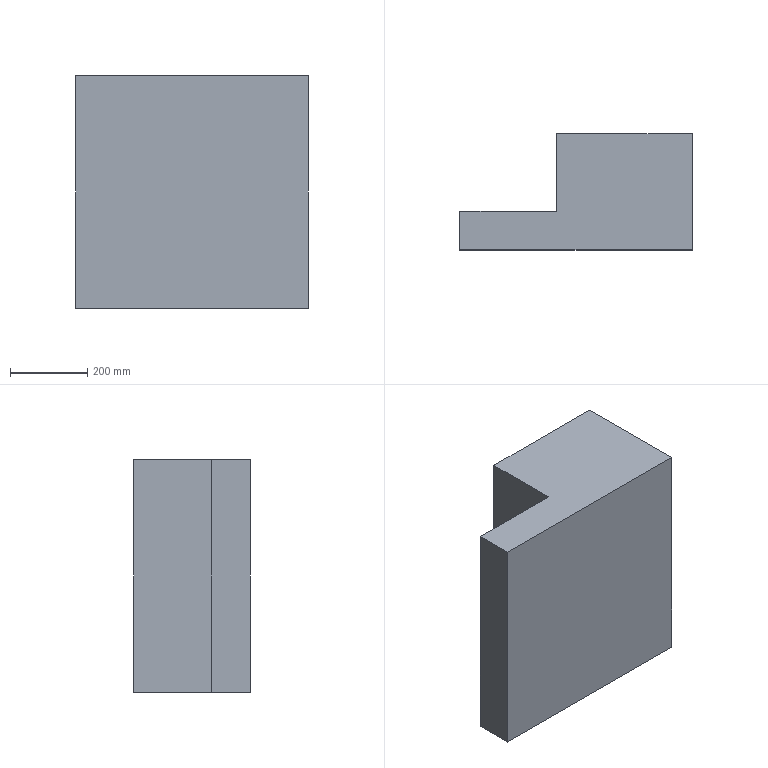Part | SolidWorks | features Extrusion 1 | 1 solid | 8 faces | box 600 x 300 x 600 mm | volume 78000000 mm3 | plane 8
STEP:
#1=CARTESIAN_POINT('',(0.,0.,-300.));
#2=VERTEX_POINT('',#1);
#3=CARTESIAN_POINT('',(600.,0.,-300.));
#4=VERTEX_POINT('',#3);
#5=CARTESIAN_POINT('',(600.,0.,-300.));
#6=DIRECTION('',(1.,0.,0.));
#7=VECTOR('',#6,1000.);
#8=LINE('',#5,#7);
#9=EDGE_CURVE('',#2,#4,#8,.T.);
#10=ORIENTED_EDGE('',*,*,#9,.T.);
#11=CARTESIAN_POINT('',(600.,0.,300.));
#12=VERTEX_POINT('',#11);
#13=CARTESIAN_POINT('',(600.,0.,300.));
#14=DIRECTION('',(0.,0.,-1.));
#15=VECTOR('',#14,1000.);
#16=LINE('',#13,#15);
#17=EDGE_CURVE('',#12,#4,#16,.T.);
#18=ORIENTED_EDGE('',*,*,#17,.F.);
#19=CARTESIAN_POINT('',(0.,0.,300.));
#20=VERTEX_POINT('',#19);
#21=CARTESIAN_POINT('',(600.,0.,300.));
#22=DIRECTION('',(1.,0.,0.));
#23=VECTOR('',#22,1000.);
#24=LINE('',#21,#23);
#25=EDGE_CURVE('',#20,#12,#24,.T.);
#26=ORIENTED_EDGE('',*,*,#25,.F.);
#27=CARTESIAN_POINT('',(0.,0.,300.));
#28=DIRECTION('',(0.,0.,-1.));
#29=VECTOR('',#28,1000.);
#30=LINE('',#27,#29);
#31=EDGE_CURVE('',#20,#2,#30,.T.);
#32=ORIENTED_EDGE('',*,*,#31,.T.);
#33=EDGE_LOOP('',(#10,#18,#26,#32));
#34=FACE_OUTER_BOUND('',#33,.T.);
#35=CARTESIAN_POINT('',(600.,0.,300.));
#36=DIRECTION('',(0.,1.,0.));
#37=DIRECTION('',(-1.,0.,0.));
#38=AXIS2_PLACEMENT_3D('',#35,#36,#37);
#39=PLANE('',#38);
#40=ADVANCED_FACE('',(#34),#39,.F.);
#41=CARTESIAN_POINT('',(600.,300.,-300.));
#42=VERTEX_POINT('',#41);
#43=CARTESIAN_POINT('',(600.,300.,-300.));
#44=DIRECTION('',(0.,1.,0.));
#45=VECTOR('',#44,1000.);
#46=LINE('',#43,#45);
#47=EDGE_CURVE('',#4,#42,#46,.T.);
#48=ORIENTED_EDGE('',*,*,#47,.T.);
#49=CARTESIAN_POINT('',(600.,300.,300.));
#50=VERTEX_POINT('',#49);
#51=CARTESIAN_POINT('',(600.,300.,300.));
#52=DIRECTION('',(0.,0.,-1.));
#53=VECTOR('',#52,1000.);
#54=LINE('',#51,#53);
#55=EDGE_CURVE('',#50,#42,#54,.T.);
#56=ORIENTED_EDGE('',*,*,#55,.F.);
#57=CARTESIAN_POINT('',(600.,300.,300.));
#58=DIRECTION('',(0.,1.,0.));
#59=VECTOR('',#58,1000.);
#60=LINE('',#57,#59);
#61=EDGE_CURVE('',#12,#50,#60,.T.);
#62=ORIENTED_EDGE('',*,*,#61,.F.);
#63=ORIENTED_EDGE('',*,*,#17,.T.);
#64=EDGE_LOOP('',(#48,#56,#62,#63));
#65=FACE_OUTER_BOUND('',#64,.T.);
#66=CARTESIAN_POINT('',(600.,300.,300.));
#67=DIRECTION('',(-1.,0.,0.));
#68=DIRECTION('',(0.,0.,1.));
#69=AXIS2_PLACEMENT_3D('',#66,#67,#68);
#70=PLANE('',#69);
#71=ADVANCED_FACE('',(#65),#70,.F.);
#72=CARTESIAN_POINT('',(250.,300.,-300.));
#73=VERTEX_POINT('',#72);
#74=CARTESIAN_POINT('',(250.,300.,-300.));
#75=DIRECTION('',(-1.,0.,0.));
#76=VECTOR('',#75,1000.);
#77=LINE('',#74,#76);
#78=EDGE_CURVE('',#42,#73,#77,.T.);
#79=ORIENTED_EDGE('',*,*,#78,.T.);
#80=CARTESIAN_POINT('',(250.,300.,300.));
#81=VERTEX_POINT('',#80);
#82=CARTESIAN_POINT('',(250.,300.,300.));
#83=DIRECTION('',(0.,0.,-1.));
#84=VECTOR('',#83,1000.);
#85=LINE('',#82,#84);
#86=EDGE_CURVE('',#81,#73,#85,.T.);
#87=ORIENTED_EDGE('',*,*,#86,.F.);
#88=CARTESIAN_POINT('',(250.,300.,300.));
#89=DIRECTION('',(-1.,0.,0.));
#90=VECTOR('',#89,1000.);
#91=LINE('',#88,#90);
#92=EDGE_CURVE('',#50,#81,#91,.T.);
#93=ORIENTED_EDGE('',*,*,#92,.F.);
#94=ORIENTED_EDGE('',*,*,#55,.T.);
#95=EDGE_LOOP('',(#79,#87,#93,#94));
#96=FACE_OUTER_BOUND('',#95,.T.);
#97=CARTESIAN_POINT('',(250.,300.,300.));
#98=DIRECTION('',(0.,-1.,0.));
#99=DIRECTION('',(0.,0.,-1.));
#100=AXIS2_PLACEMENT_3D('',#97,#98,#99);
#101=PLANE('',#100);
#102=ADVANCED_FACE('',(#96),#101,.F.);
#103=CARTESIAN_POINT('',(250.,100.,-300.));
#104=VERTEX_POINT('',#103);
#105=CARTESIAN_POINT('',(250.,100.,-300.));
#106=DIRECTION('',(0.,-1.,0.));
#107=VECTOR('',#106,1000.);
#108=LINE('',#105,#107);
#109=EDGE_CURVE('',#73,#104,#108,.T.);
#110=ORIENTED_EDGE('',*,*,#109,.T.);
#111=CARTESIAN_POINT('',(250.,100.,300.));
#112=VERTEX_POINT('',#111);
#113=CARTESIAN_POINT('',(250.,100.,300.));
#114=DIRECTION('',(0.,0.,-1.));
#115=VECTOR('',#114,1000.);
#116=LINE('',#113,#115);
#117=EDGE_CURVE('',#112,#104,#116,.T.);
#118=ORIENTED_EDGE('',*,*,#117,.F.);
#119=CARTESIAN_POINT('',(250.,100.,300.));
#120=DIRECTION('',(0.,-1.,0.));
#121=VECTOR('',#120,1000.);
#122=LINE('',#119,#121);
#123=EDGE_CURVE('',#81,#112,#122,.T.);
#124=ORIENTED_EDGE('',*,*,#123,.F.);
#125=ORIENTED_EDGE('',*,*,#86,.T.);
#126=EDGE_LOOP('',(#110,#118,#124,#125));
#127=FACE_OUTER_BOUND('',#126,.T.);
#128=CARTESIAN_POINT('',(250.,100.,300.));
#129=DIRECTION('',(1.,0.,0.));
#130=DIRECTION('',(0.,0.,-1.));
#131=AXIS2_PLACEMENT_3D('',#128,#129,#130);
#132=PLANE('',#131);
#133=ADVANCED_FACE('',(#127),#132,.F.);
#134=CARTESIAN_POINT('',(0.,100.,-300.));
#135=VERTEX_POINT('',#134);
#136=CARTESIAN_POINT('',(0.,100.,-300.));
#137=DIRECTION('',(-1.,0.,0.));
#138=VECTOR('',#137,1000.);
#139=LINE('',#136,#138);
#140=EDGE_CURVE('',#104,#135,#139,.T.);
#141=ORIENTED_EDGE('',*,*,#140,.T.);
#142=CARTESIAN_POINT('',(0.,100.,300.));
#143=VERTEX_POINT('',#142);
#144=CARTESIAN_POINT('',(0.,100.,300.));
#145=DIRECTION('',(0.,0.,-1.));
#146=VECTOR('',#145,1000.);
#147=LINE('',#144,#146);
#148=EDGE_CURVE('',#143,#135,#147,.T.);
#149=ORIENTED_EDGE('',*,*,#148,.F.);
#150=CARTESIAN_POINT('',(0.,100.,300.));
#151=DIRECTION('',(-1.,0.,0.));
#152=VECTOR('',#151,1000.);
#153=LINE('',#150,#152);
#154=EDGE_CURVE('',#112,#143,#153,.T.);
#155=ORIENTED_EDGE('',*,*,#154,.F.);
#156=ORIENTED_EDGE('',*,*,#117,.T.);
#157=EDGE_LOOP('',(#141,#149,#155,#156));
#158=FACE_OUTER_BOUND('',#157,.T.);
#159=CARTESIAN_POINT('',(0.,100.,300.));
#160=DIRECTION('',(0.,-1.,0.));
#161=DIRECTION('',(0.,0.,-1.));
#162=AXIS2_PLACEMENT_3D('',#159,#160,#161);
#163=PLANE('',#162);
#164=ADVANCED_FACE('',(#158),#163,.F.);
#165=CARTESIAN_POINT('',(0.,0.,-300.));
#166=DIRECTION('',(0.,-1.,0.));
#167=VECTOR('',#166,1000.);
#168=LINE('',#165,#167);
#169=EDGE_CURVE('',#135,#2,#168,.T.);
#170=ORIENTED_EDGE('',*,*,#169,.T.);
#171=ORIENTED_EDGE('',*,*,#31,.F.);
#172=CARTESIAN_POINT('',(0.,0.,300.));
#173=DIRECTION('',(0.,-1.,0.));
#174=VECTOR('',#173,1000.);
#175=LINE('',#172,#174);
#176=EDGE_CURVE('',#143,#20,#175,.T.);
#177=ORIENTED_EDGE('',*,*,#176,.F.);
#178=ORIENTED_EDGE('',*,*,#148,.T.);
#179=EDGE_LOOP('',(#170,#171,#177,#178));
#180=FACE_OUTER_BOUND('',#179,.T.);
#181=CARTESIAN_POINT('',(0.,0.,300.));
#182=DIRECTION('',(1.,0.,0.));
#183=DIRECTION('',(0.,0.,-1.));
#184=AXIS2_PLACEMENT_3D('',#181,#182,#183);
#185=PLANE('',#184);
#186=ADVANCED_FACE('',(#180),#185,.F.);
#187=ORIENTED_EDGE('',*,*,#25,.T.);
#188=ORIENTED_EDGE('',*,*,#61,.T.);
#189=ORIENTED_EDGE('',*,*,#92,.T.);
#190=ORIENTED_EDGE('',*,*,#123,.T.);
#191=ORIENTED_EDGE('',*,*,#154,.T.);
#192=ORIENTED_EDGE('',*,*,#176,.T.);
#193=EDGE_LOOP('',(#187,#188,#189,#190,#191,#192));
#194=FACE_OUTER_BOUND('',#193,.T.);
#195=CARTESIAN_POINT('',(0.,0.,300.));
#196=DIRECTION('',(0.,0.,-1.));
#197=DIRECTION('',(-1.,0.,0.));
#198=AXIS2_PLACEMENT_3D('',#195,#196,#197);
#199=PLANE('',#198);
#200=ADVANCED_FACE('',(#194),#199,.F.);
#201=ORIENTED_EDGE('',*,*,#9,.F.);
#202=ORIENTED_EDGE('',*,*,#169,.F.);
#203=ORIENTED_EDGE('',*,*,#140,.F.);
#204=ORIENTED_EDGE('',*,*,#109,.F.);
#205=ORIENTED_EDGE('',*,*,#78,.F.);
#206=ORIENTED_EDGE('',*,*,#47,.F.);
#207=EDGE_LOOP('',(#201,#202,#203,#204,#205,#206));
#208=FACE_OUTER_BOUND('',#207,.T.);
#209=CARTESIAN_POINT('',(0.,0.,-300.));
#210=DIRECTION('',(0.,0.,-1.));
#211=DIRECTION('',(-1.,0.,0.));
#212=AXIS2_PLACEMENT_3D('',#209,#210,#211);
#213=PLANE('',#212);
#214=ADVANCED_FACE('',(#208),#213,.T.);
#215=CLOSED_SHELL('',(#40,#71,#102,#133,#164,#186,#200,#214));
#216=MANIFOLD_SOLID_BREP('',#215);
#217=CARTESIAN_POINT('',(0.,0.,0.));
#218=DIRECTION('',(0.,0.,1.));
#219=DIRECTION('',(1.,0.,0.));
#220=AXIS2_PLACEMENT_3D('',#217,#218,#219);
#221=(LENGTH_UNIT()NAMED_UNIT(*)SI_UNIT(.MILLI.,.METRE.));
#222=UNCERTAINTY_MEASURE_WITH_UNIT(LENGTH_MEASURE(0.00001),#221,'','');
#223=(NAMED_UNIT(*)PLANE_ANGLE_UNIT()SI_UNIT($,.RADIAN.));
#224=(NAMED_UNIT(*)SI_UNIT($,.STERADIAN.)SOLID_ANGLE_UNIT());
#225=(GEOMETRIC_REPRESENTATION_CONTEXT(3)GLOBAL_UNCERTAINTY_ASSIGNED_CONTEXT((#222))GLOBAL_UNIT_ASSIGNED_CONTEXT((#221,#223,#224))REPRESENTATION_CONTEXT('',''));
#226=ADVANCED_BREP_SHAPE_REPRESENTATION('',(#216,#220),#225);